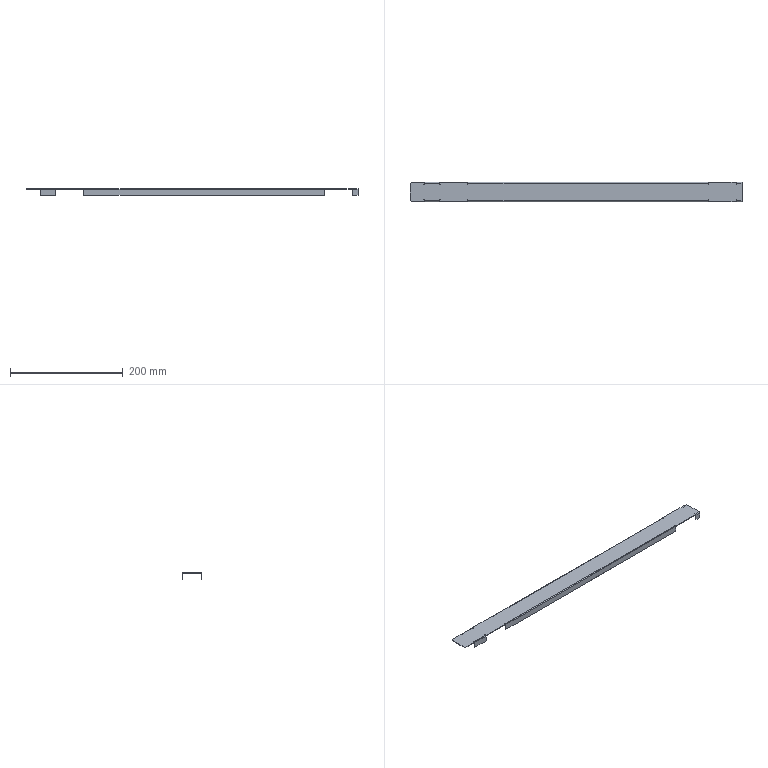Part | SolidWorks | features SMBaseFlange 2, Chamfer 1, Cut 1, EdgeFlange 1, FlatPattern 1, ICE 1, MirrorPattern 1, SheetMetal 1 | 1 solid | 96 faces | box 590 x 34 x 12 mm | volume 29992 mm3 | plane 84 | cylinder 12 | commonest cylinder face diameters 0.4 x6 2.4 x6